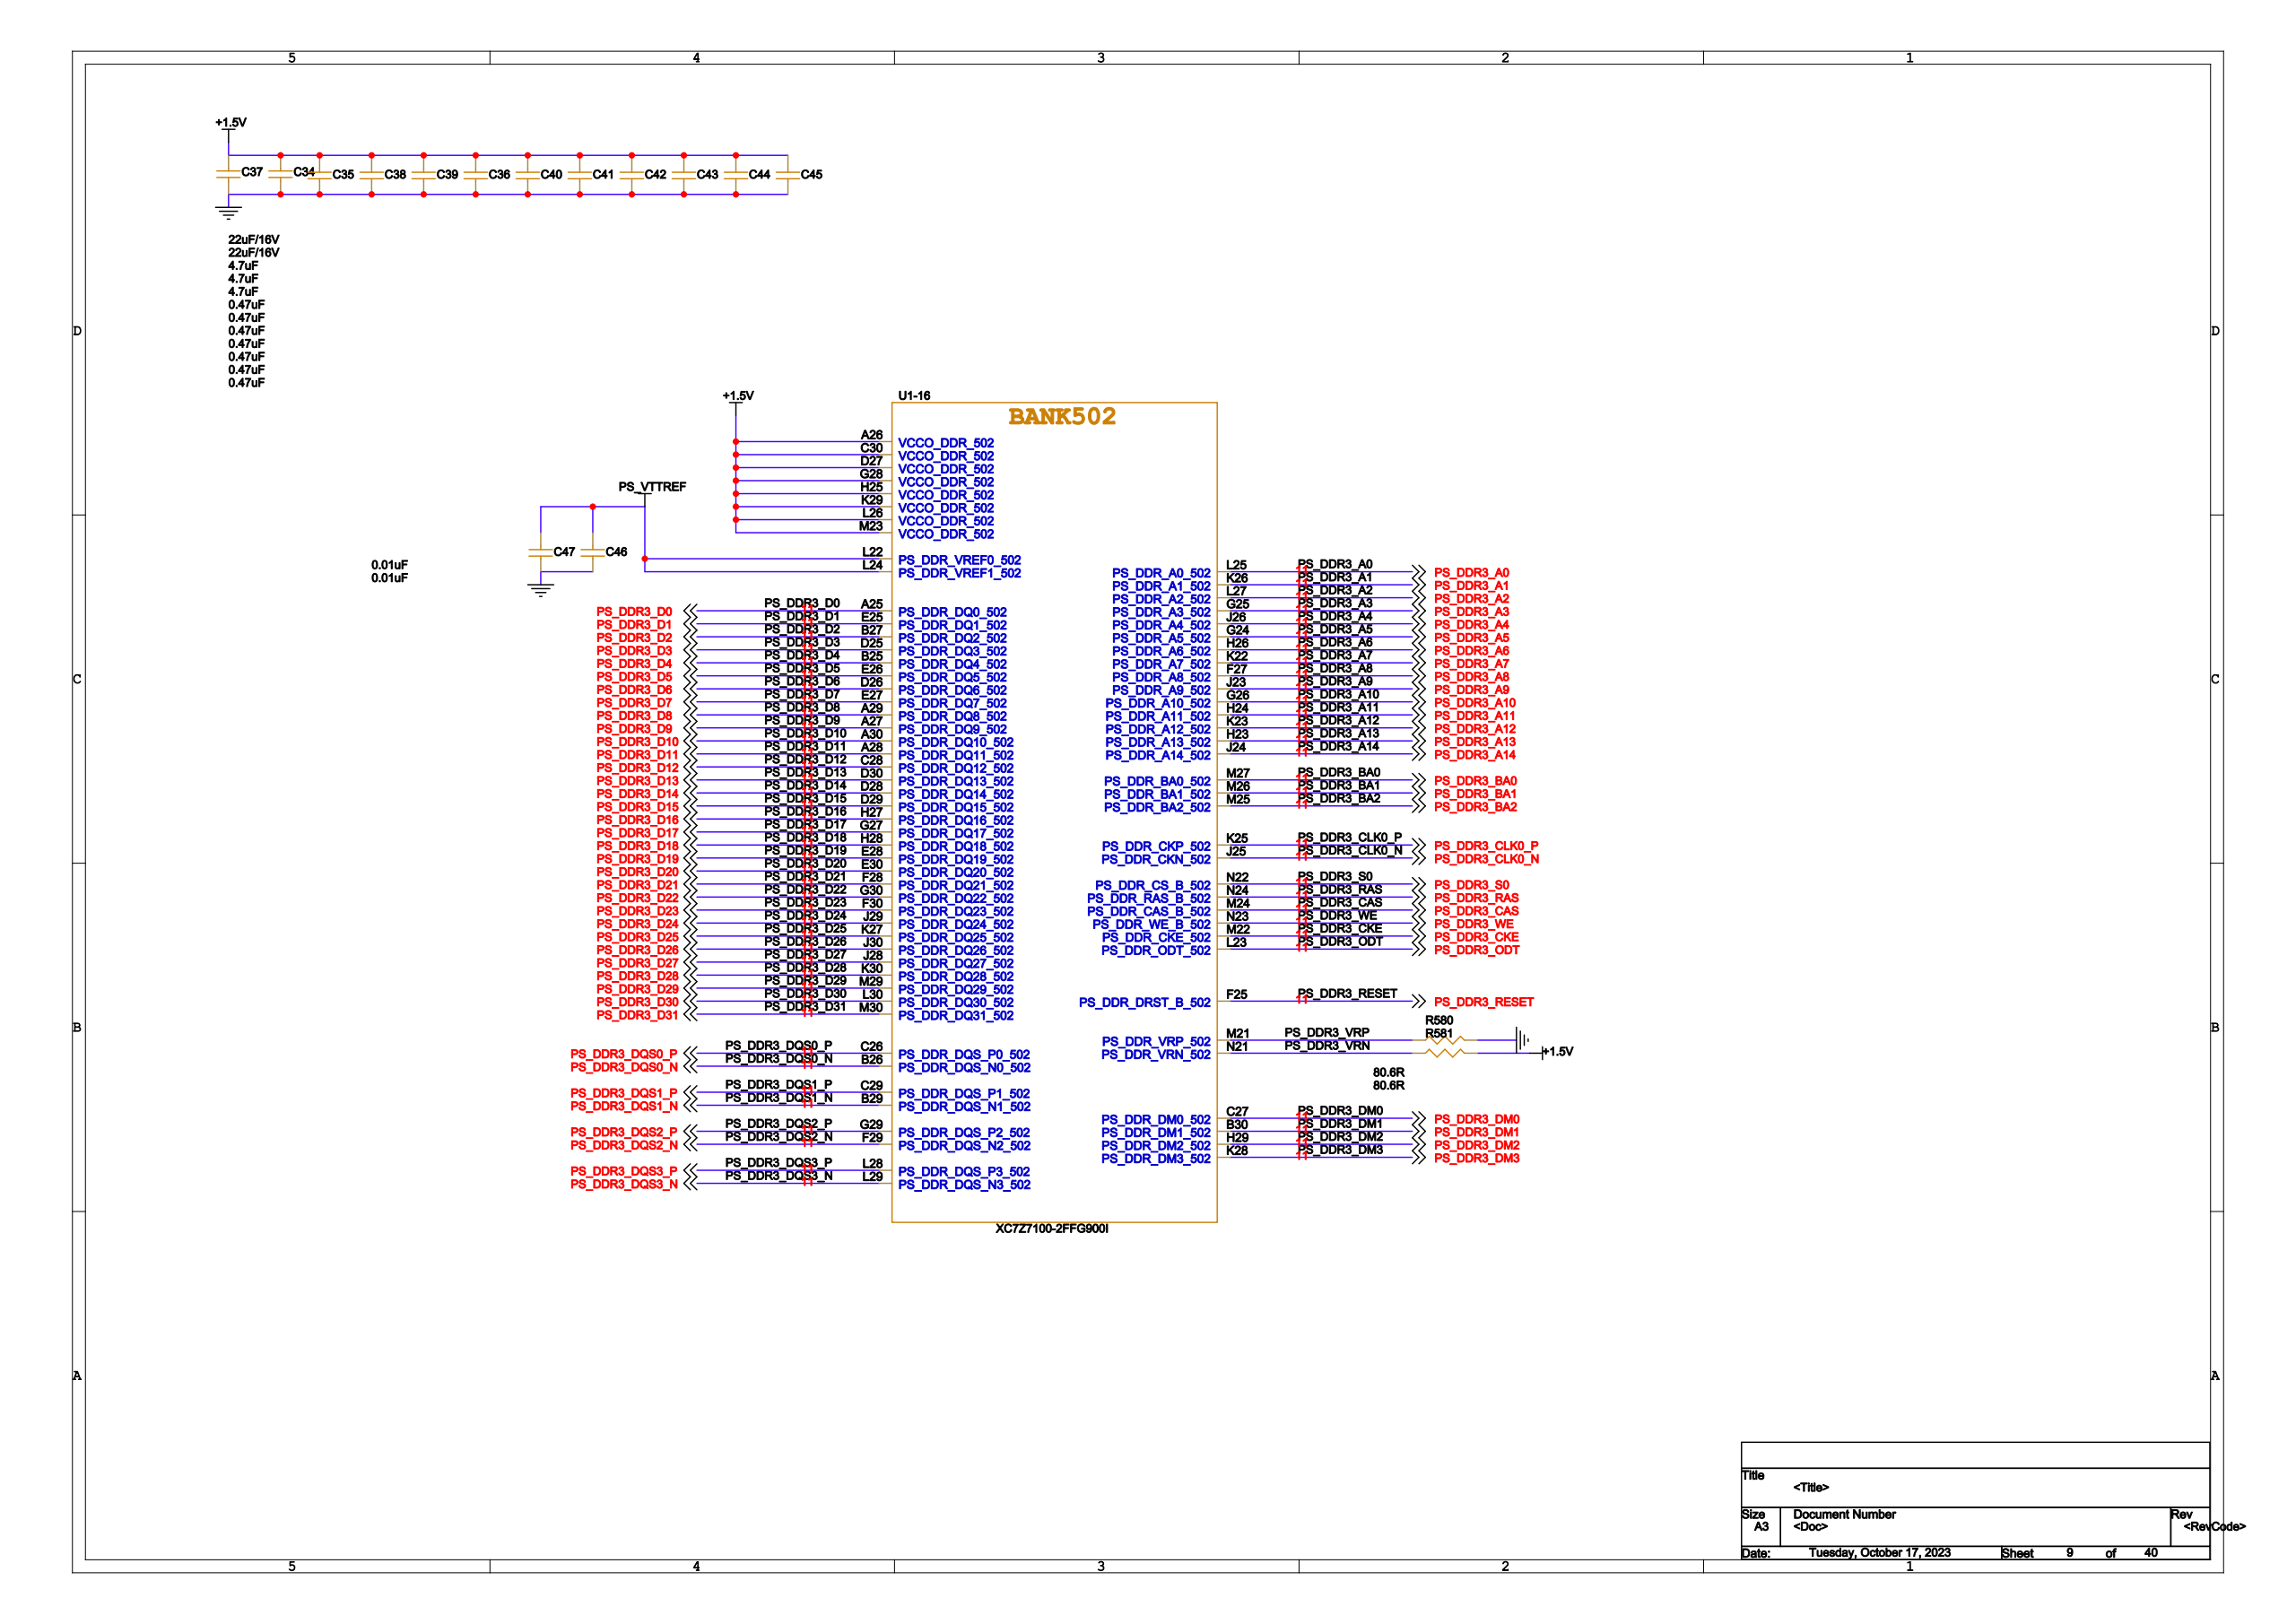Circuit board | Cadence Allegro | 1793 parts | 1223 nets | one sheet of the schematic
Parts on this sheet (reference | value | footprint):
C34 | 22uF/16V | C0603
C35 | 4.7uF | C0402
C36 | 0.47uF | C0402
C37 | 22uF/16V | C0603
C38 | 4.7uF | C0402
C39 | 4.7uF | C0402
C40 | 0.47uF | C0402
C41 | 0.47uF | C0402
C42 | 0.47uF | C0402
C43 | 0.47uF | C0402
C44 | 0.47uF | C0402
C45 | 0.47uF | C0402
C46 | 0.01uF | C0402
C47 | 0.01uF | C0402
R580 | 80.6R | R0402
R581 | 80.6R | R0402
Nets of these parts (net: part-pin ...):
GND: C34-2 C35-1 C36-1 C37-2 C38-1 C39-1 C40-1 C41-1 C42-1 C43-1 C44-1 C45-1 C46-1 C47-1 R580-1
+1.5V: C34-1 C35-2 C36-2 C37-1 C38-2 C39-2 C40-2 C41-2 C42-2 C43-2 C44-2 C45-2 R581-1
PS_VTTREF: C46-2 C47-2
PS_DDR3_VRP: R580-2
PS_DDR3_VRN: R581-2